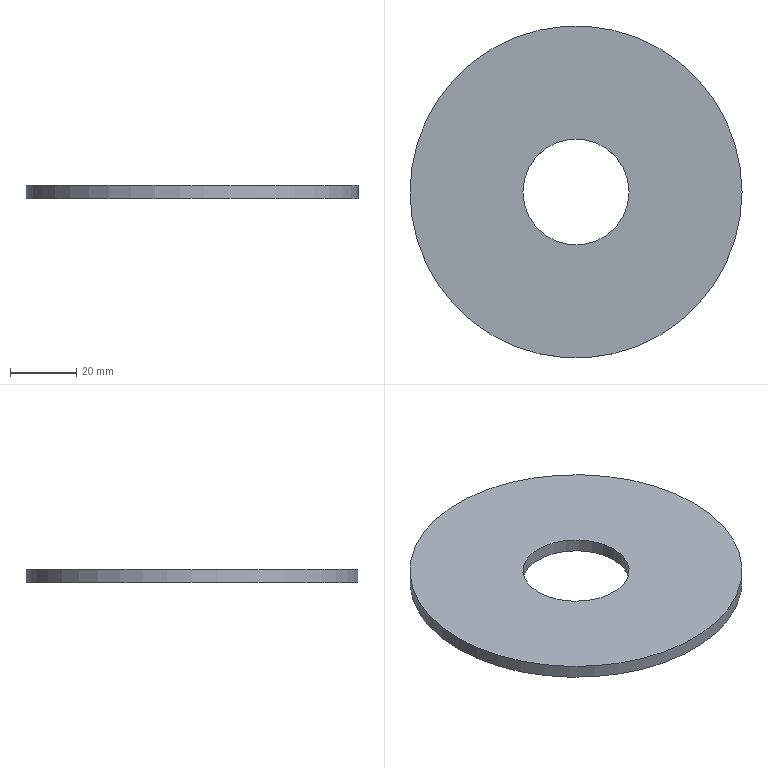Part | STEP file | Slotted wheel end cap 2 | 1 solid | 4 faces | box 100 x 100 x 4 mm | volume 28199 mm3 | plane 2 | cylinder 2 | commonest cylinder face diameters 32 x1 100 x1
STEP:
#1=CARTESIAN_POINT('',(50.,0.,4.));
#2=VERTEX_POINT('',#1);
#3=CARTESIAN_POINT('',(0.,0.,4.));
#4=DIRECTION('',(0.,0.,1.));
#5=DIRECTION('',(1.,0.,0.));
#6=AXIS2_PLACEMENT_3D('',#3,#4,#5);
#7=CIRCLE('',#6,50.);
#8=EDGE_CURVE('',#2,#2,#7,.T.);
#9=ORIENTED_EDGE('',*,*,#8,.T.);
#10=EDGE_LOOP('',(#9));
#11=FACE_OUTER_BOUND('',#10,.T.);
#12=CARTESIAN_POINT('',(16.,0.,4.));
#13=VERTEX_POINT('',#12);
#14=CARTESIAN_POINT('',(0.,0.,4.));
#15=DIRECTION('',(0.,0.,1.));
#16=DIRECTION('',(1.,0.,0.));
#17=AXIS2_PLACEMENT_3D('',#14,#15,#16);
#18=CIRCLE('',#17,16.);
#19=EDGE_CURVE('',#13,#13,#18,.T.);
#20=ORIENTED_EDGE('',*,*,#19,.F.);
#21=EDGE_LOOP('',(#20));
#22=FACE_BOUND('',#21,.T.);
#23=CARTESIAN_POINT('',(0.,0.,4.));
#24=DIRECTION('',(0.,0.,1.));
#25=DIRECTION('',(1.,0.,0.));
#26=AXIS2_PLACEMENT_3D('',#23,#24,#25);
#27=PLANE('',#26);
#28=ADVANCED_FACE('',(#11,#22),#27,.T.);
#29=CARTESIAN_POINT('',(50.,0.,0.));
#30=VERTEX_POINT('',#29);
#31=CARTESIAN_POINT('',(0.,0.,0.));
#32=DIRECTION('',(0.,0.,1.));
#33=DIRECTION('',(1.,0.,0.));
#34=AXIS2_PLACEMENT_3D('',#31,#32,#33);
#35=CIRCLE('',#34,50.);
#36=EDGE_CURVE('',#30,#30,#35,.T.);
#37=ORIENTED_EDGE('',*,*,#36,.F.);
#38=EDGE_LOOP('',(#37));
#39=FACE_OUTER_BOUND('',#38,.T.);
#40=CARTESIAN_POINT('',(16.,0.,0.));
#41=VERTEX_POINT('',#40);
#42=CARTESIAN_POINT('',(0.,0.,0.));
#43=DIRECTION('',(0.,0.,1.));
#44=DIRECTION('',(1.,0.,0.));
#45=AXIS2_PLACEMENT_3D('',#42,#43,#44);
#46=CIRCLE('',#45,16.);
#47=EDGE_CURVE('',#41,#41,#46,.T.);
#48=ORIENTED_EDGE('',*,*,#47,.T.);
#49=EDGE_LOOP('',(#48));
#50=FACE_BOUND('',#49,.T.);
#51=CARTESIAN_POINT('',(0.,0.,0.));
#52=DIRECTION('',(0.,0.,1.));
#53=DIRECTION('',(1.,0.,0.));
#54=AXIS2_PLACEMENT_3D('',#51,#52,#53);
#55=PLANE('',#54);
#56=ADVANCED_FACE('',(#39,#50),#55,.F.);
#57=ORIENTED_EDGE('',*,*,#8,.F.);
#58=EDGE_LOOP('',(#57));
#59=FACE_OUTER_BOUND('',#58,.T.);
#60=ORIENTED_EDGE('',*,*,#36,.T.);
#61=EDGE_LOOP('',(#60));
#62=FACE_OUTER_BOUND('',#61,.T.);
#63=CARTESIAN_POINT('',(0.,0.,4.));
#64=DIRECTION('',(0.,0.,-1.));
#65=DIRECTION('',(-1.,0.,0.));
#66=AXIS2_PLACEMENT_3D('',#63,#64,#65);
#67=CYLINDRICAL_SURFACE('',#66,50.);
#68=ADVANCED_FACE('',(#59,#62),#67,.T.);
#69=ORIENTED_EDGE('',*,*,#19,.T.);
#70=EDGE_LOOP('',(#69));
#71=FACE_OUTER_BOUND('',#70,.T.);
#72=ORIENTED_EDGE('',*,*,#47,.F.);
#73=EDGE_LOOP('',(#72));
#74=FACE_OUTER_BOUND('',#73,.T.);
#75=CARTESIAN_POINT('',(0.,0.,4.));
#76=DIRECTION('',(0.,0.,-1.));
#77=DIRECTION('',(-1.,0.,0.));
#78=AXIS2_PLACEMENT_3D('',#75,#76,#77);
#79=CYLINDRICAL_SURFACE('',#78,16.);
#80=ADVANCED_FACE('',(#71,#74),#79,.F.);
#81=CLOSED_SHELL('',(#28,#56,#68,#80));
#82=MANIFOLD_SOLID_BREP('',#81);
#83=CARTESIAN_POINT('',(0.,0.,0.));
#84=DIRECTION('',(0.,0.,1.));
#85=DIRECTION('',(1.,0.,0.));
#86=AXIS2_PLACEMENT_3D('',#83,#84,#85);
#87=(LENGTH_UNIT()NAMED_UNIT(*)SI_UNIT(.MILLI.,.METRE.));
#88=UNCERTAINTY_MEASURE_WITH_UNIT(LENGTH_MEASURE(0.00001),#87,'','');
#89=(NAMED_UNIT(*)PLANE_ANGLE_UNIT()SI_UNIT($,.RADIAN.));
#90=(NAMED_UNIT(*)SI_UNIT($,.STERADIAN.)SOLID_ANGLE_UNIT());
#91=(GEOMETRIC_REPRESENTATION_CONTEXT(3)GLOBAL_UNCERTAINTY_ASSIGNED_CONTEXT((#88))GLOBAL_UNIT_ASSIGNED_CONTEXT((#87,#89,#90))REPRESENTATION_CONTEXT('',''));
#92=ADVANCED_BREP_SHAPE_REPRESENTATION('',(#82,#86),#91);